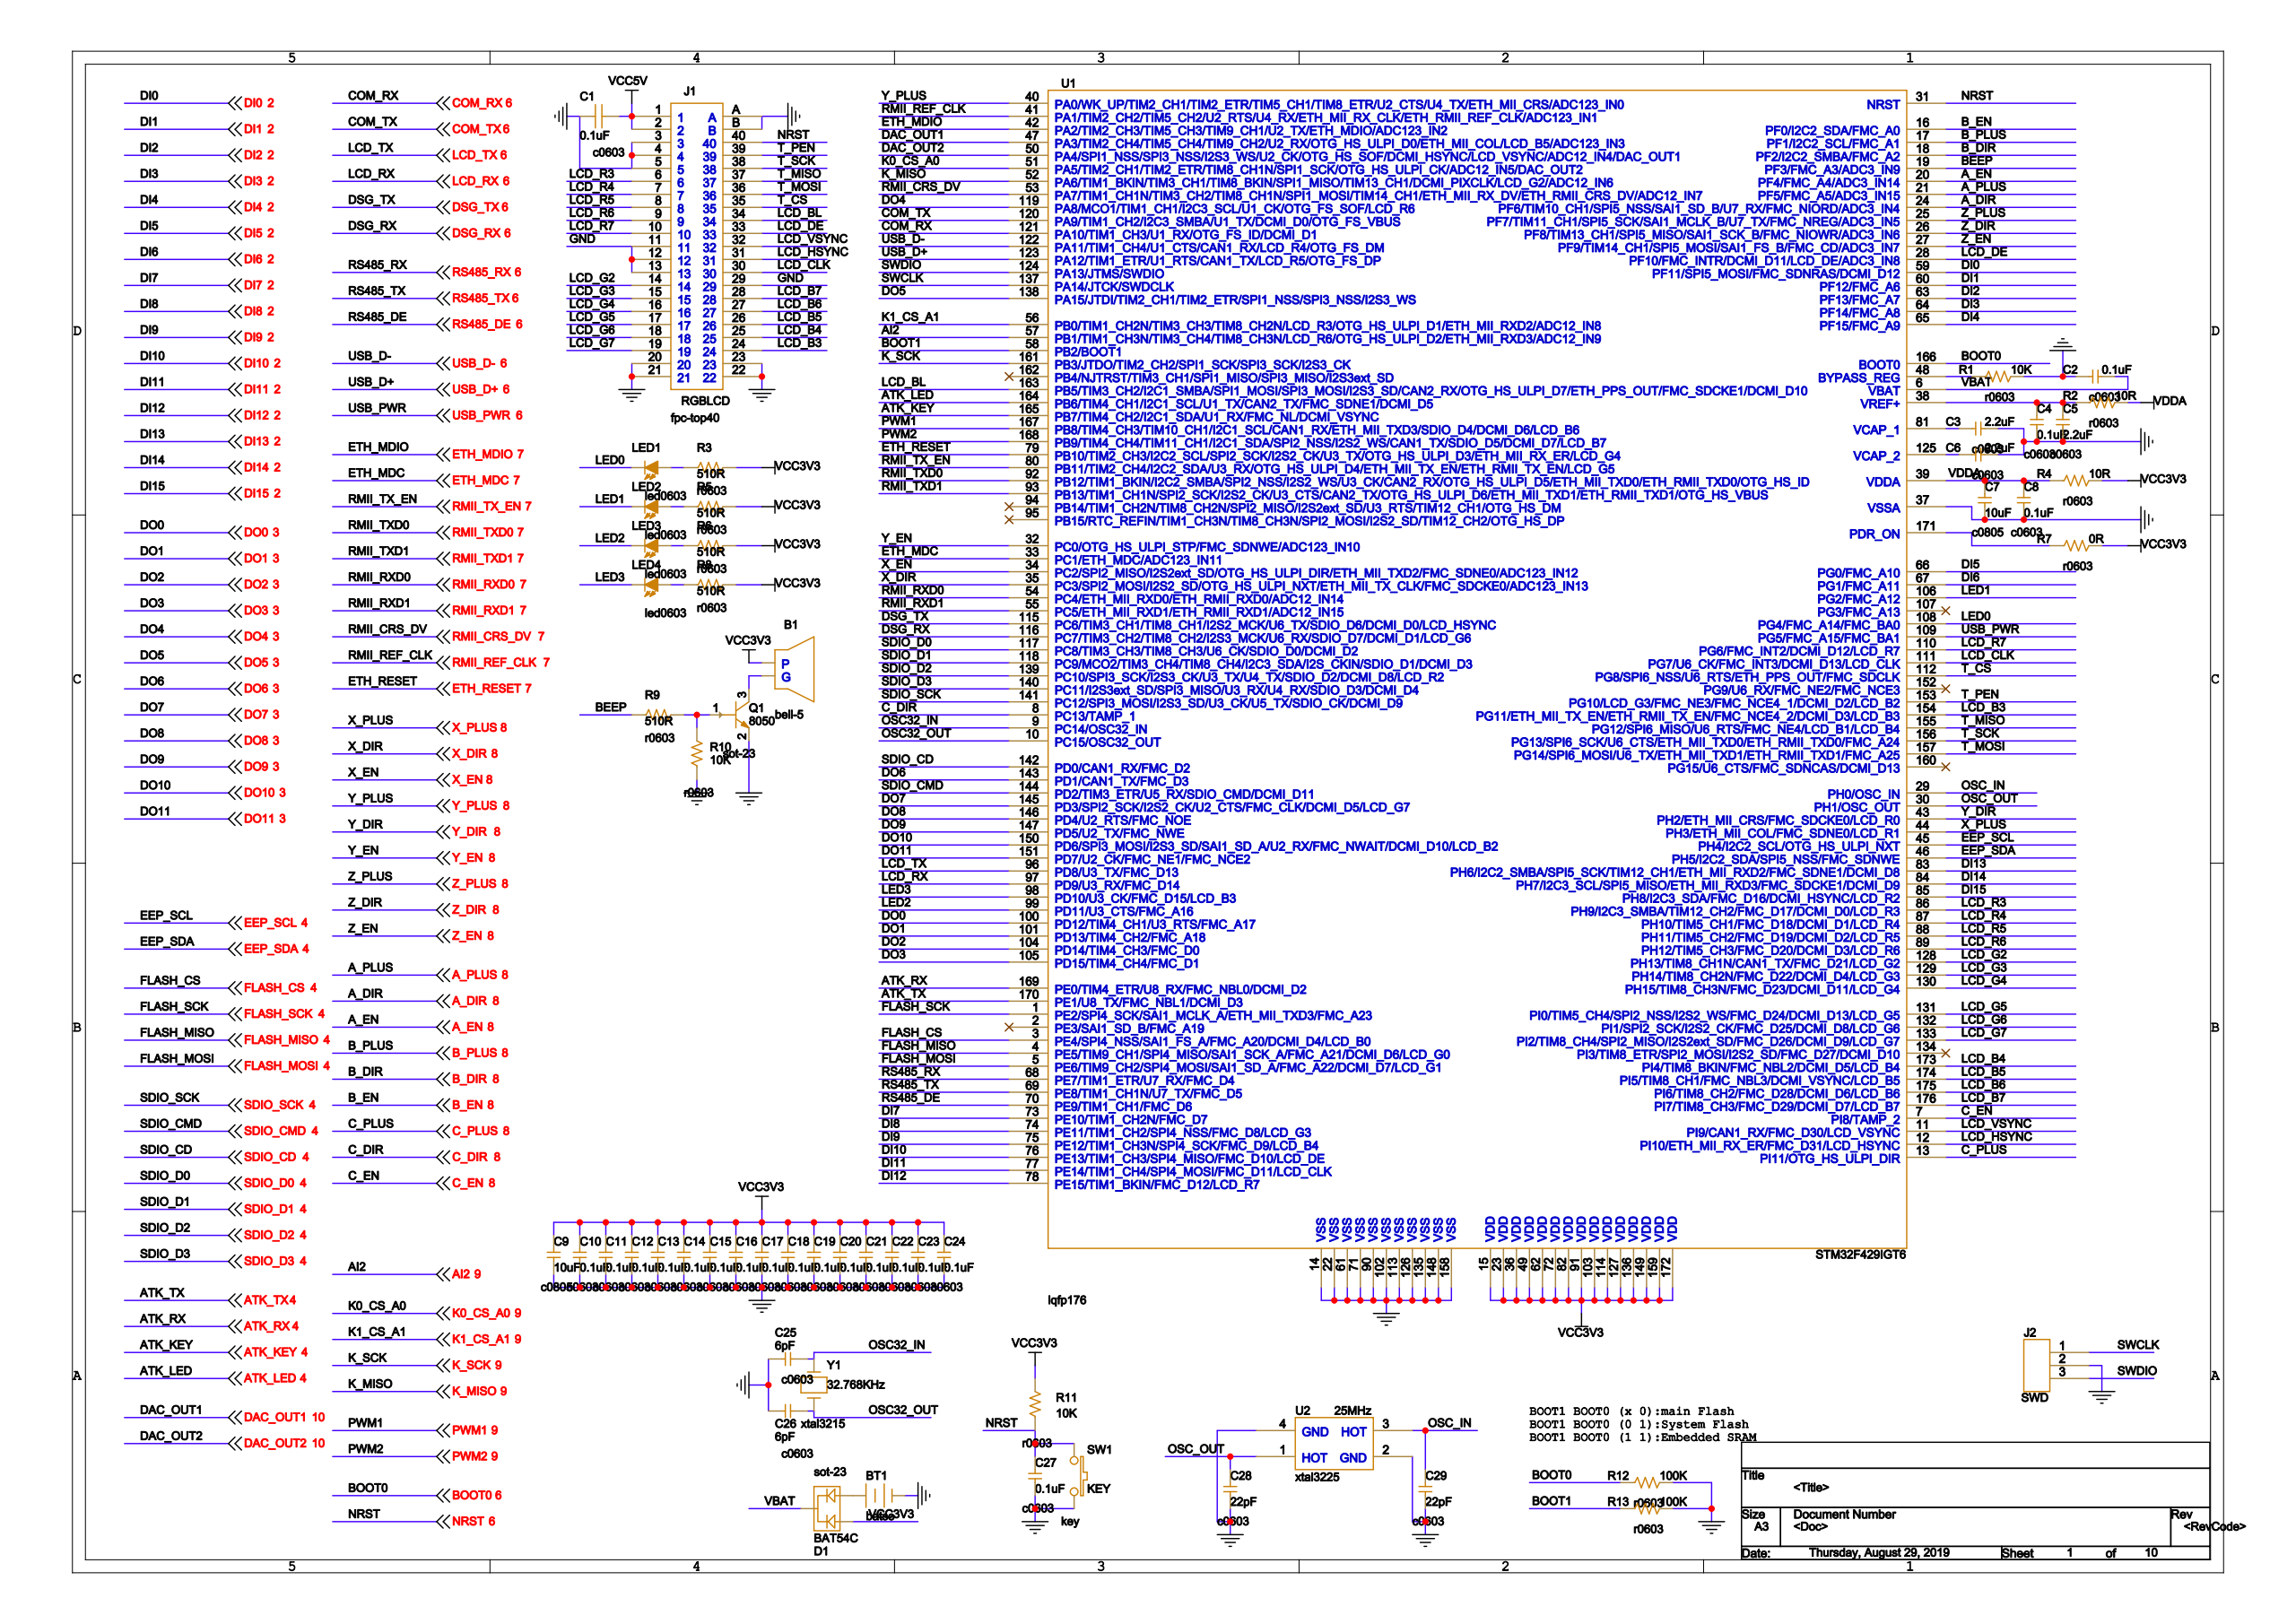Circuit board | Cadence Allegro | 380 parts | 375 nets | one sheet of the schematic
Parts on this sheet (reference | value | footprint):
B1 | BEEP | BELL-5
BT1 | BATTERY | BATSO
C1 | 0.1uF | C0603
C2 | 0.1uF | C0603
C3 | 2.2uF | C0603
C4 | 0.1uF | C0603
C5 | 2.2uF | C0603
C6 | 2.2uF | C0603
C7 | 10uF | C0805
C8 | 0.1uF | C0603
C9 | 10uF | C0805
C10 | 0.1uF | C0603
C11 | 0.1uF | C0603
C12 | 0.1uF | C0603
C13 | 0.1uF | C0603
C14 | 0.1uF | C0603
C15 | 0.1uF | C0603
C16 | 0.1uF | C0603
C17 | 0.1uF | C0603
C18 | 0.1uF | C0603
C19 | 0.1uF | C0603
C20 | 0.1uF | C0603
C21 | 0.1uF | C0603
C22 | 0.1uF | C0603
C23 | 0.1uF | C0603
C24 | 0.1uF | C0603
C25 | 6pF | C0603
C26 | 6pF | C0603
C27 | 0.1uF | C0603
C28 | 22pF | C0603
C29 | 22pF | C0603
D1 | BAT54C | SOT-23
J1 | RGBLCD | FPC-TOP40
J2 | SWD | CON2_54X1X3
LED1 | LED | LED0603
LED2 | LED | LED0603
LED3 | LED | LED0603
LED4 | LED | LED0603
Q1 | 8050 | SOT-23
R1 | 10K | R0603
R2 | 10R | R0603
R3 | 510R | R0603
R4 | 10R | R0603
R5 | 510R | R0603
R6 | 510R | R0603
R8 | 510R | R0603
R9 | 510R | R0603
R10 | 10K | R0603
R11 | 10K | R0603
R12 | 100K | R0603
R13 | 100K | R0603
SW1 | KEY | KEY
U1 | STM32F429IGT6 | LQFP176
U2 | 25MHz | XTAL3225
Y1 | 32.768KHz | XTAL3215
Nets of these parts (net: part-pin ...):
GND: BT1-2 C1-1 C2-1 C3-2 C4-2 C5-2 C6-2 C7-2 C8-2 C9-1 C10-1 C11-1 C12-1 C13-1 C14-1 C15-1 C16-1 C17-1 C18-1 C19-1 C20-1 C21-1 C22-1 C23-1 C24-1 C25-2 C26-2 C27-1 C28-2 C29-2 J2-2 Q1-2 R1-2 R10-1 R12-2 R13-2 SW1-2 U2-2 U2-4 J1-3 J1-4 J1-5 J1-11 J1-12 J1-13 J1-20 J1-21 J1-22 J1-23 J1-29 J1-A J1-B U1-14 U1-22 U1-37 U1-61 U1-71 U1-90 U1-102 U1-113 U1-126 U1-135 U1-148 U1-158
SWCLK: J2-1 U1-137
SWDIO: J2-3 U1-124
VCC3V3: B1-1 C9-2 C10-2 C11-2 C12-2 C13-2 C14-2 C15-2 C16-2 C17-2 C18-2 C19-2 C20-2 C21-2 C22-2 C23-2 C24-2 D1-2 R3-2 R4-2 R5-2 R6-2 R8-2 R11-2 U1-15 U1-23 U1-36 U1-49 U1-62 U1-72 U1-82 U1-91 U1-103 U1-114 U1-127 U1-136 U1-149 U1-159 U1-172
DI3: U1-64
DI2: U1-63
DI1: U1-60
DI0: U1-59
DI11: U1-77
DI10: U1-76
DI9: U1-75
DI8: U1-74
DI7: U1-73
DI6: U1-67
DI5: U1-66
DI4: U1-65
DI15: U1-85
DI14: U1-84
DI13: U1-83
DI12: U1-78
DO3: U1-105
DO2: U1-104
DO1: U1-101
DO0: U1-100
DO7: U1-145
DO6: U1-143
DO5: U1-138
DO4: U1-119
DO10: U1-150
DO9: U1-147
DO8: U1-146
COM_TX: U1-120
COM_RX: U1-121
SDIO_CD: U1-142
SDIO_D3: U1-140
SDIO_SCK: U1-141
SDIO_CMD: U1-144
SDIO_D0: U1-117
SDIO_D1: U1-118
SDIO_D2: U1-139
VCC5V: C1-2 J1-1 J1-2
USB_D-: U1-122
USB_D+: U1-123
USB_PWR: U1-109
AI2: U1-57
K0_CS_A0: U1-51
K1_CS_A1: U1-56
EEP_SCL: U1-45
EEP_SDA: U1-46
FLASH_CS: U1-3
FLASH_SCK: U1-1
FLASH_MOSI: U1-5
FLASH_MISO: U1-4
LCD_RX: U1-97
DSG_RX: U1-116
LCD_TX: U1-96
DSG_TX: U1-115
RS485_DE: U1-70
RS485_TX: U1-69
RS485_RX: U1-68
DAC_OUT1: U1-47
DAC_OUT2: U1-50
N1655153: B1-2 Q1-3
N15685230: BT1-1 D1-1
VBAT: C2-2 D1-3 U1-6
NRST: C27-2 R11-1 SW1-1 J1-40 U1-31
N1561296: C4-1 C5-1 R2-1 U1-38
VDDA: C7-1 C8-1 R2-2 R4-1 U1-39
OSC32_IN: C25-1 Y1-2 U1-9
OSC32_OUT: C26-1 Y1-1 U1-10
OSC_OUT: C28-1 U2-1 U1-30
OSC_IN: C29-1 U2-3 U1-29
N1561488: C3-1 U1-81
N1561490: C6-1 U1-125
LCD_R7: J1-10 U1-110
LCD_G2: J1-14 U1-128
LCD_G3: J1-15 U1-129
LCD_G4: J1-16 U1-130
LCD_G5: J1-17 U1-131
LCD_G6: J1-18 U1-132
LCD_G7: J1-19 U1-133
LCD_B3: J1-24 U1-154
LCD_B4: J1-25 U1-173
LCD_B5: J1-26 U1-174
LCD_B6: J1-27 U1-175
LCD_B7: J1-28 U1-176
LCD_CLK: J1-30 U1-111
LCD_HSYNC: J1-31 U1-12
LCD_VSYNC: J1-32 U1-11
LCD_DE: J1-33 U1-28
LCD_BL: J1-34 U1-163
T_CS: J1-35 U1-112
T_MOSI: J1-36 U1-157
T_MISO: J1-37 U1-155
T_SCK: J1-38 U1-156
T_PEN: J1-39 U1-153
LCD_R3: J1-6 U1-86
LCD_R4: J1-7 U1-87
LCD_R5: J1-8 U1-88
LCD_R6: J1-9 U1-89
ATK_TX: U1-170
ATK_RX: U1-169
ATK_KEY: U1-165
ATK_LED: U1-164
N1653736: LED1-1 R3-1
LED0: LED1-2 U1-108
N1653871: LED2-1 R5-1
LED1: LED2-2 U1-106
N1655804: LED3-1 R6-1
LED2: LED3-2 U1-99
N1655926: LED4-1 R8-1
LED3: LED4-2 U1-98
B_DIR: U1-18
B_PLUS: U1-17
B_EN: U1-16
C_DIR: U1-8
C_PLUS: U1-13
C_EN: U1-7
N1654172: Q1-1 R9-2 R10-2
PWM1: U1-167
N1560879: R1-1 U1-48
PWM2: U1-168
BOOT0: R12-1 U1-166
BOOT1: R13-1 U1-58
ETH_MDIO: U1-42
BEEP: R9-1 U1-19
Z_PLUS: U1-25
Z_DIR: U1-26
A_PLUS: U1-21
A_DIR: U1-24
X_PLUS: U1-44
X_DIR: U1-35
Y_PLUS: U1-40
Y_DIR: U1-43
RMII_REF_CLK: U1-41
K_MISO: U1-52
RMII_CRS_DV: U1-53
ETH_RESET: U1-79
RMII_TX_EN: U1-80
RMII_TXD0: U1-92
RMII_TXD1: U1-93
K_SCK: U1-161
Y_EN: U1-32
ETH_MDC: U1-33
X_EN: U1-34
RMII_RXD0: U1-54
RMII_RXD1: U1-55
DO11: U1-151
A_EN: U1-20
Z_EN: U1-27